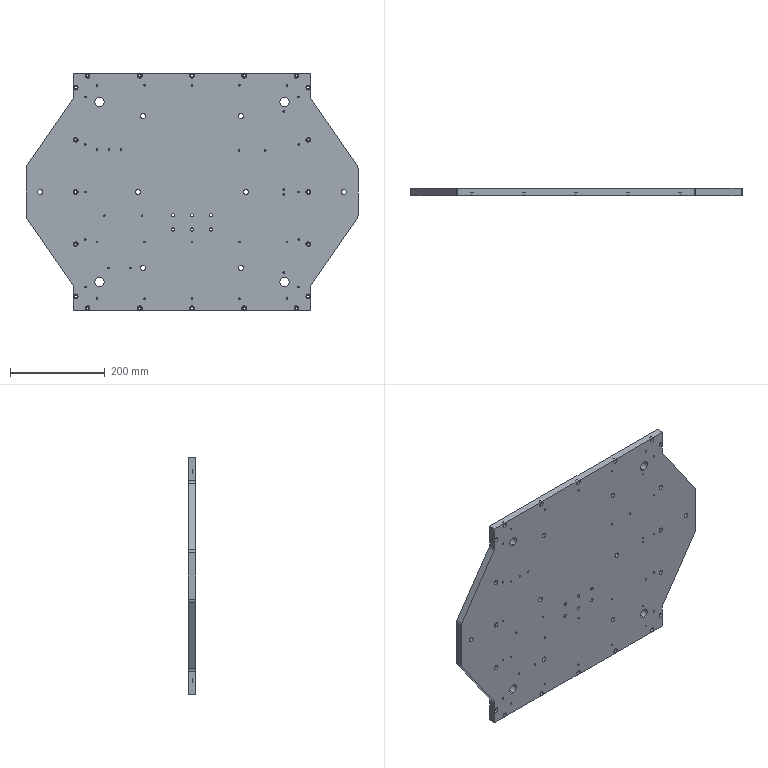Part | SolidWorks | features HoleWzd 5, Cut 1, Extrusion 1, Fillet 1, ICE 1 | 1 solid | 234 faces | box 700 x 15 x 500 mm | volume 4450228 mm3 | cylinder 200 | plane 34 | commonest cylinder face diameters 3.3 x76 5.5 x40 9.9 x40 11 x16 20 x16 6.8 x12